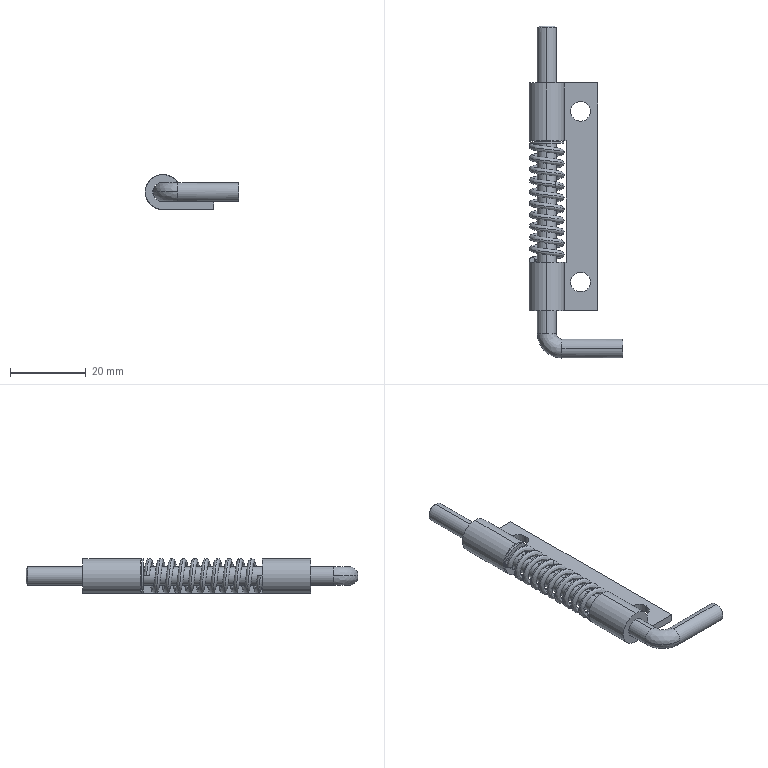Part | STEP file | CL225-3-Z Shengjiu spring plunger-dddeger | 3 solids | 49 faces | box 24.6 x 87.5 x 9.2 mm | volume 4748 mm3 | cylinder 20 | plane 19 | spline 8 | cone 2 | commonest cylinder face diameters 5.2 x7 5 x4 9.2 x4 6 x3 9 x2